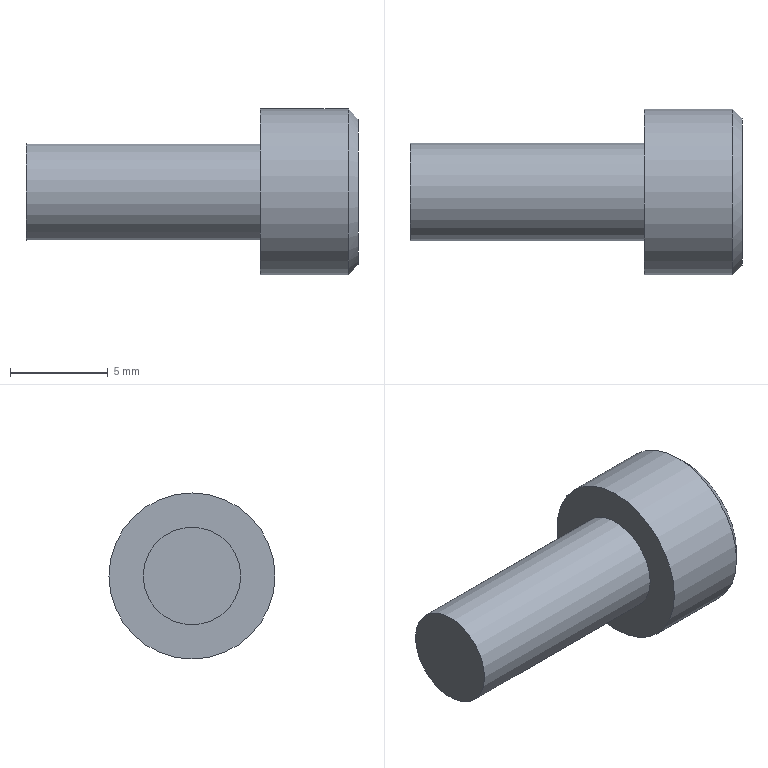Part | NX | features 5003_313_CB5-12 2 | 1 solid | 19 faces | box 17 x 8.5 x 8.5 mm | volume 476.463 mm3 | plane 15 | cylinder 2 | cone 2 | commonest cylinder face diameters 5 x1 8.5 x1
STEP:
#1=CARTESIAN_POINT('',(228.825,-163.25,-78.));
#2=VERTEX_POINT('',#1);
#3=CARTESIAN_POINT('',(228.825,-167.,-78.));
#4=DIRECTION('',(-1.,0.,0.));
#5=DIRECTION('',(0.,1.,0.));
#6=AXIS2_PLACEMENT_3D('',#3,#4,#5);
#7=CIRCLE('',#6,3.75);
#8=EDGE_CURVE('',#2,#2,#7,.F.);
#9=ORIENTED_EDGE('',*,*,#8,.T.);
#10=EDGE_LOOP('',(#9));
#11=FACE_BOUND('',#10,.T.);
#12=CARTESIAN_POINT('',(228.825,-167.,-75.691));
#13=VERTEX_POINT('',#12);
#14=CARTESIAN_POINT('',(228.825,-169.,-76.845));
#15=VERTEX_POINT('',#14);
#16=CARTESIAN_POINT('',(228.825,-167.,-75.691));
#17=DIRECTION('',(0.,-0.866,-0.5));
#18=VECTOR('',#17,1000.);
#19=LINE('',#16,#18);
#20=EDGE_CURVE('',#13,#15,#19,.T.);
#21=ORIENTED_EDGE('',*,*,#20,.F.);
#22=CARTESIAN_POINT('',(228.825,-165.,-76.845));
#23=VERTEX_POINT('',#22);
#24=CARTESIAN_POINT('',(228.825,-165.,-76.845));
#25=DIRECTION('',(0.,-0.866,0.5));
#26=VECTOR('',#25,1000.);
#27=LINE('',#24,#26);
#28=EDGE_CURVE('',#23,#13,#27,.T.);
#29=ORIENTED_EDGE('',*,*,#28,.F.);
#30=CARTESIAN_POINT('',(228.825,-165.,-79.155));
#31=VERTEX_POINT('',#30);
#32=CARTESIAN_POINT('',(228.825,-165.,-79.155));
#33=DIRECTION('',(0.,0.,1.));
#34=VECTOR('',#33,1000.);
#35=LINE('',#32,#34);
#36=EDGE_CURVE('',#31,#23,#35,.T.);
#37=ORIENTED_EDGE('',*,*,#36,.F.);
#38=CARTESIAN_POINT('',(228.825,-167.,-80.309));
#39=VERTEX_POINT('',#38);
#40=CARTESIAN_POINT('',(228.825,-167.,-80.309));
#41=DIRECTION('',(0.,0.866,0.5));
#42=VECTOR('',#41,1000.);
#43=LINE('',#40,#42);
#44=EDGE_CURVE('',#39,#31,#43,.T.);
#45=ORIENTED_EDGE('',*,*,#44,.F.);
#46=CARTESIAN_POINT('',(228.825,-169.,-79.155));
#47=VERTEX_POINT('',#46);
#48=CARTESIAN_POINT('',(228.825,-169.,-79.155));
#49=DIRECTION('',(0.,0.866,-0.5));
#50=VECTOR('',#49,1000.);
#51=LINE('',#48,#50);
#52=EDGE_CURVE('',#47,#39,#51,.T.);
#53=ORIENTED_EDGE('',*,*,#52,.F.);
#54=CARTESIAN_POINT('',(228.825,-169.,-76.845));
#55=DIRECTION('',(0.,0.,-1.));
#56=VECTOR('',#55,1000.);
#57=LINE('',#54,#56);
#58=EDGE_CURVE('',#15,#47,#57,.T.);
#59=ORIENTED_EDGE('',*,*,#58,.F.);
#60=EDGE_LOOP('',(#21,#29,#37,#45,#53,#59));
#61=FACE_BOUND('',#60,.T.);
#62=CARTESIAN_POINT('',(228.825,-167.,-82.25));
#63=DIRECTION('',(-1.,0.,0.));
#64=DIRECTION('',(0.,1.,0.));
#65=AXIS2_PLACEMENT_3D('',#62,#63,#64);
#66=PLANE('',#65);
#67=ADVANCED_FACE('',(#11,#61),#66,.F.);
#68=CARTESIAN_POINT('',(211.825,-169.5,-78.));
#69=VERTEX_POINT('',#68);
#70=CARTESIAN_POINT('',(211.825,-167.,-78.));
#71=DIRECTION('',(1.,0.,0.));
#72=DIRECTION('',(0.,-1.,0.));
#73=AXIS2_PLACEMENT_3D('',#70,#71,#72);
#74=CIRCLE('',#73,2.5);
#75=EDGE_CURVE('',#69,#69,#74,.T.);
#76=ORIENTED_EDGE('',*,*,#75,.F.);
#77=EDGE_LOOP('',(#76));
#78=FACE_BOUND('',#77,.T.);
#79=CARTESIAN_POINT('',(211.825,-167.,-78.));
#80=DIRECTION('',(1.,0.,0.));
#81=DIRECTION('',(0.,-1.,0.));
#82=AXIS2_PLACEMENT_3D('',#79,#80,#81);
#83=PLANE('',#82);
#84=ADVANCED_FACE('',(#78),#83,.F.);
#85=CARTESIAN_POINT('',(223.825,-169.5,-78.));
#86=VERTEX_POINT('',#85);
#87=CARTESIAN_POINT('',(223.825,-167.,-78.));
#88=DIRECTION('',(1.,0.,0.));
#89=DIRECTION('',(0.,-1.,0.));
#90=AXIS2_PLACEMENT_3D('',#87,#88,#89);
#91=CIRCLE('',#90,2.5);
#92=EDGE_CURVE('',#86,#86,#91,.T.);
#93=ORIENTED_EDGE('',*,*,#92,.F.);
#94=EDGE_LOOP('',(#93));
#95=FACE_BOUND('',#94,.T.);
#96=ORIENTED_EDGE('',*,*,#75,.T.);
#97=EDGE_LOOP('',(#96));
#98=FACE_BOUND('',#97,.T.);
#99=CARTESIAN_POINT('',(228.825,-167.,-78.));
#100=DIRECTION('',(1.,0.,0.));
#101=DIRECTION('',(0.,-1.,0.));
#102=AXIS2_PLACEMENT_3D('',#99,#100,#101);
#103=CYLINDRICAL_SURFACE('',#102,2.5);
#104=ADVANCED_FACE('',(#95,#98),#103,.T.);
#105=CARTESIAN_POINT('',(223.825,-171.25,-78.));
#106=VERTEX_POINT('',#105);
#107=CARTESIAN_POINT('',(223.825,-167.,-78.));
#108=DIRECTION('',(1.,0.,0.));
#109=DIRECTION('',(0.,-1.,0.));
#110=AXIS2_PLACEMENT_3D('',#107,#108,#109);
#111=CIRCLE('',#110,4.25);
#112=EDGE_CURVE('',#106,#106,#111,.T.);
#113=ORIENTED_EDGE('',*,*,#112,.F.);
#114=EDGE_LOOP('',(#113));
#115=FACE_BOUND('',#114,.T.);
#116=ORIENTED_EDGE('',*,*,#92,.T.);
#117=EDGE_LOOP('',(#116));
#118=FACE_BOUND('',#117,.T.);
#119=CARTESIAN_POINT('',(223.825,-167.,-80.5));
#120=DIRECTION('',(1.,0.,0.));
#121=DIRECTION('',(0.,-1.,0.));
#122=AXIS2_PLACEMENT_3D('',#119,#120,#121);
#123=PLANE('',#122);
#124=ADVANCED_FACE('',(#115,#118),#123,.F.);
#125=CARTESIAN_POINT('',(228.325,-162.75,-78.));
#126=VERTEX_POINT('',#125);
#127=CARTESIAN_POINT('',(228.325,-167.,-78.));
#128=DIRECTION('',(-1.,0.,0.));
#129=DIRECTION('',(0.,1.,0.));
#130=AXIS2_PLACEMENT_3D('',#127,#128,#129);
#131=CIRCLE('',#130,4.25);
#132=EDGE_CURVE('',#126,#126,#131,.T.);
#133=ORIENTED_EDGE('',*,*,#132,.T.);
#134=EDGE_LOOP('',(#133));
#135=FACE_BOUND('',#134,.T.);
#136=ORIENTED_EDGE('',*,*,#112,.T.);
#137=EDGE_LOOP('',(#136));
#138=FACE_BOUND('',#137,.T.);
#139=CARTESIAN_POINT('',(228.825,-167.,-78.));
#140=DIRECTION('',(1.,0.,0.));
#141=DIRECTION('',(0.,-1.,0.));
#142=AXIS2_PLACEMENT_3D('',#139,#140,#141);
#143=CYLINDRICAL_SURFACE('',#142,4.25);
#144=ADVANCED_FACE('',(#135,#138),#143,.T.);
#145=ORIENTED_EDGE('',*,*,#132,.F.);
#146=EDGE_LOOP('',(#145));
#147=FACE_BOUND('',#146,.T.);
#148=ORIENTED_EDGE('',*,*,#8,.F.);
#149=EDGE_LOOP('',(#148));
#150=FACE_BOUND('',#149,.T.);
#151=CARTESIAN_POINT('',(228.825,-167.,-78.));
#152=DIRECTION('',(-1.,0.,0.));
#153=DIRECTION('',(0.,1.,0.));
#154=AXIS2_PLACEMENT_3D('',#151,#152,#153);
#155=CONICAL_SURFACE('',#154,3.75,0.7854);
#156=ADVANCED_FACE('',(#147,#150),#155,.T.);
#157=CARTESIAN_POINT('',(226.325,-165.,-76.845));
#158=VERTEX_POINT('',#157);
#159=CARTESIAN_POINT('',(226.325,-166.,-76.268));
#160=VERTEX_POINT('',#159);
#161=CARTESIAN_POINT('',(226.325,-165.,-76.845));
#162=DIRECTION('',(0.,-0.866,0.5));
#163=VECTOR('',#162,1000.);
#164=LINE('',#161,#163);
#165=EDGE_CURVE('',#158,#160,#164,.T.);
#166=ORIENTED_EDGE('',*,*,#165,.F.);
#167=CARTESIAN_POINT('',(226.325,-165.,-76.845));
#168=DIRECTION('',(1.,0.,0.));
#169=VECTOR('',#168,1000.);
#170=LINE('',#167,#169);
#171=EDGE_CURVE('',#158,#23,#170,.T.);
#172=ORIENTED_EDGE('',*,*,#171,.T.);
#173=ORIENTED_EDGE('',*,*,#28,.T.);
#174=CARTESIAN_POINT('',(226.325,-167.,-75.691));
#175=VERTEX_POINT('',#174);
#176=CARTESIAN_POINT('',(226.325,-167.,-75.691));
#177=DIRECTION('',(1.,0.,0.));
#178=VECTOR('',#177,1000.);
#179=LINE('',#176,#178);
#180=EDGE_CURVE('',#175,#13,#179,.T.);
#181=ORIENTED_EDGE('',*,*,#180,.F.);
#182=CARTESIAN_POINT('',(226.325,-165.,-76.845));
#183=DIRECTION('',(0.,-0.866,0.5));
#184=VECTOR('',#183,1000.);
#185=LINE('',#182,#184);
#186=EDGE_CURVE('',#160,#175,#185,.T.);
#187=ORIENTED_EDGE('',*,*,#186,.F.);
#188=EDGE_LOOP('',(#166,#172,#173,#181,#187));
#189=FACE_BOUND('',#188,.T.);
#190=CARTESIAN_POINT('',(226.325,-165.,-76.845));
#191=DIRECTION('',(0.,0.5,0.866));
#192=DIRECTION('',(0.,0.866,-0.5));
#193=AXIS2_PLACEMENT_3D('',#190,#191,#192);
#194=PLANE('',#193);
#195=ADVANCED_FACE('',(#189),#194,.F.);
#196=CARTESIAN_POINT('',(226.325,-165.,-79.155));
#197=VERTEX_POINT('',#196);
#198=CARTESIAN_POINT('',(226.325,-165.,-78.));
#199=VERTEX_POINT('',#198);
#200=CARTESIAN_POINT('',(226.325,-165.,-79.155));
#201=DIRECTION('',(0.,0.,1.));
#202=VECTOR('',#201,1000.);
#203=LINE('',#200,#202);
#204=EDGE_CURVE('',#197,#199,#203,.T.);
#205=ORIENTED_EDGE('',*,*,#204,.F.);
#206=CARTESIAN_POINT('',(226.325,-165.,-79.155));
#207=DIRECTION('',(1.,0.,0.));
#208=VECTOR('',#207,1000.);
#209=LINE('',#206,#208);
#210=EDGE_CURVE('',#197,#31,#209,.T.);
#211=ORIENTED_EDGE('',*,*,#210,.T.);
#212=ORIENTED_EDGE('',*,*,#36,.T.);
#213=ORIENTED_EDGE('',*,*,#171,.F.);
#214=CARTESIAN_POINT('',(226.325,-165.,-79.155));
#215=DIRECTION('',(0.,0.,1.));
#216=VECTOR('',#215,1000.);
#217=LINE('',#214,#216);
#218=EDGE_CURVE('',#199,#158,#217,.T.);
#219=ORIENTED_EDGE('',*,*,#218,.F.);
#220=EDGE_LOOP('',(#205,#211,#212,#213,#219));
#221=FACE_BOUND('',#220,.T.);
#222=CARTESIAN_POINT('',(226.325,-165.,-79.155));
#223=DIRECTION('',(0.,1.,0.));
#224=DIRECTION('',(1.,0.,0.));
#225=AXIS2_PLACEMENT_3D('',#222,#223,#224);
#226=PLANE('',#225);
#227=ADVANCED_FACE('',(#221),#226,.F.);
#228=CARTESIAN_POINT('',(226.325,-167.,-80.309));
#229=VERTEX_POINT('',#228);
#230=CARTESIAN_POINT('',(226.325,-166.,-79.732));
#231=VERTEX_POINT('',#230);
#232=CARTESIAN_POINT('',(226.325,-167.,-80.309));
#233=DIRECTION('',(0.,0.866,0.5));
#234=VECTOR('',#233,1000.);
#235=LINE('',#232,#234);
#236=EDGE_CURVE('',#229,#231,#235,.T.);
#237=ORIENTED_EDGE('',*,*,#236,.F.);
#238=CARTESIAN_POINT('',(226.325,-167.,-80.309));
#239=DIRECTION('',(1.,0.,0.));
#240=VECTOR('',#239,1000.);
#241=LINE('',#238,#240);
#242=EDGE_CURVE('',#229,#39,#241,.T.);
#243=ORIENTED_EDGE('',*,*,#242,.T.);
#244=ORIENTED_EDGE('',*,*,#44,.T.);
#245=ORIENTED_EDGE('',*,*,#210,.F.);
#246=CARTESIAN_POINT('',(226.325,-167.,-80.309));
#247=DIRECTION('',(0.,0.866,0.5));
#248=VECTOR('',#247,1000.);
#249=LINE('',#246,#248);
#250=EDGE_CURVE('',#231,#197,#249,.T.);
#251=ORIENTED_EDGE('',*,*,#250,.F.);
#252=EDGE_LOOP('',(#237,#243,#244,#245,#251));
#253=FACE_BOUND('',#252,.T.);
#254=CARTESIAN_POINT('',(226.325,-167.,-80.309));
#255=DIRECTION('',(0.,0.5,-0.866));
#256=DIRECTION('',(0.,-0.866,-0.5));
#257=AXIS2_PLACEMENT_3D('',#254,#255,#256);
#258=PLANE('',#257);
#259=ADVANCED_FACE('',(#253),#258,.F.);
#260=CARTESIAN_POINT('',(226.325,-169.,-79.155));
#261=VERTEX_POINT('',#260);
#262=CARTESIAN_POINT('',(226.325,-168.,-79.732));
#263=VERTEX_POINT('',#262);
#264=CARTESIAN_POINT('',(226.325,-169.,-79.155));
#265=DIRECTION('',(0.,0.866,-0.5));
#266=VECTOR('',#265,1000.);
#267=LINE('',#264,#266);
#268=EDGE_CURVE('',#261,#263,#267,.T.);
#269=ORIENTED_EDGE('',*,*,#268,.F.);
#270=CARTESIAN_POINT('',(226.325,-169.,-79.155));
#271=DIRECTION('',(1.,0.,0.));
#272=VECTOR('',#271,1000.);
#273=LINE('',#270,#272);
#274=EDGE_CURVE('',#261,#47,#273,.T.);
#275=ORIENTED_EDGE('',*,*,#274,.T.);
#276=ORIENTED_EDGE('',*,*,#52,.T.);
#277=ORIENTED_EDGE('',*,*,#242,.F.);
#278=CARTESIAN_POINT('',(226.325,-169.,-79.155));
#279=DIRECTION('',(0.,0.866,-0.5));
#280=VECTOR('',#279,1000.);
#281=LINE('',#278,#280);
#282=EDGE_CURVE('',#263,#229,#281,.T.);
#283=ORIENTED_EDGE('',*,*,#282,.F.);
#284=EDGE_LOOP('',(#269,#275,#276,#277,#283));
#285=FACE_BOUND('',#284,.T.);
#286=CARTESIAN_POINT('',(226.325,-169.,-79.155));
#287=DIRECTION('',(0.,-0.5,-0.866));
#288=DIRECTION('',(0.,-0.866,0.5));
#289=AXIS2_PLACEMENT_3D('',#286,#287,#288);
#290=PLANE('',#289);
#291=ADVANCED_FACE('',(#285),#290,.F.);
#292=CARTESIAN_POINT('',(226.325,-169.,-76.845));
#293=VERTEX_POINT('',#292);
#294=CARTESIAN_POINT('',(226.325,-169.,-78.));
#295=VERTEX_POINT('',#294);
#296=CARTESIAN_POINT('',(226.325,-169.,-76.845));
#297=DIRECTION('',(0.,0.,-1.));
#298=VECTOR('',#297,1000.);
#299=LINE('',#296,#298);
#300=EDGE_CURVE('',#293,#295,#299,.T.);
#301=ORIENTED_EDGE('',*,*,#300,.F.);
#302=CARTESIAN_POINT('',(226.325,-169.,-76.845));
#303=DIRECTION('',(1.,0.,0.));
#304=VECTOR('',#303,1000.);
#305=LINE('',#302,#304);
#306=EDGE_CURVE('',#293,#15,#305,.T.);
#307=ORIENTED_EDGE('',*,*,#306,.T.);
#308=ORIENTED_EDGE('',*,*,#58,.T.);
#309=ORIENTED_EDGE('',*,*,#274,.F.);
#310=CARTESIAN_POINT('',(226.325,-169.,-76.845));
#311=DIRECTION('',(0.,0.,-1.));
#312=VECTOR('',#311,1000.);
#313=LINE('',#310,#312);
#314=EDGE_CURVE('',#295,#261,#313,.T.);
#315=ORIENTED_EDGE('',*,*,#314,.F.);
#316=EDGE_LOOP('',(#301,#307,#308,#309,#315));
#317=FACE_BOUND('',#316,.T.);
#318=CARTESIAN_POINT('',(226.325,-169.,-76.845));
#319=DIRECTION('',(0.,-1.,0.));
#320=DIRECTION('',(0.,0.,1.));
#321=AXIS2_PLACEMENT_3D('',#318,#319,#320);
#322=PLANE('',#321);
#323=ADVANCED_FACE('',(#317),#322,.F.);
#324=CARTESIAN_POINT('',(226.325,-168.,-76.268));
#325=VERTEX_POINT('',#324);
#326=CARTESIAN_POINT('',(226.325,-167.,-75.691));
#327=DIRECTION('',(0.,-0.866,-0.5));
#328=VECTOR('',#327,1000.);
#329=LINE('',#326,#328);
#330=EDGE_CURVE('',#175,#325,#329,.T.);
#331=ORIENTED_EDGE('',*,*,#330,.F.);
#332=ORIENTED_EDGE('',*,*,#180,.T.);
#333=ORIENTED_EDGE('',*,*,#20,.T.);
#334=ORIENTED_EDGE('',*,*,#306,.F.);
#335=CARTESIAN_POINT('',(226.325,-167.,-75.691));
#336=DIRECTION('',(0.,-0.866,-0.5));
#337=VECTOR('',#336,1000.);
#338=LINE('',#335,#337);
#339=EDGE_CURVE('',#325,#293,#338,.T.);
#340=ORIENTED_EDGE('',*,*,#339,.F.);
#341=EDGE_LOOP('',(#331,#332,#333,#334,#340));
#342=FACE_BOUND('',#341,.T.);
#343=CARTESIAN_POINT('',(226.325,-167.,-75.691));
#344=DIRECTION('',(0.,-0.5,0.866));
#345=DIRECTION('',(0.,0.866,0.5));
#346=AXIS2_PLACEMENT_3D('',#343,#344,#345);
#347=PLANE('',#346);
#348=ADVANCED_FACE('',(#342),#347,.F.);
#349=ORIENTED_EDGE('',*,*,#314,.T.);
#350=ORIENTED_EDGE('',*,*,#268,.T.);
#351=CARTESIAN_POINT('',(226.325,-167.,-78.));
#352=DIRECTION('',(1.,0.,0.));
#353=DIRECTION('',(0.,0.,1.));
#354=AXIS2_PLACEMENT_3D('',#351,#352,#353);
#355=CIRCLE('',#354,2.);
#356=EDGE_CURVE('',#295,#263,#355,.T.);
#357=ORIENTED_EDGE('',*,*,#356,.F.);
#358=EDGE_LOOP('',(#349,#350,#357));
#359=FACE_BOUND('',#358,.T.);
#360=CARTESIAN_POINT('',(226.325,-167.,-78.));
#361=DIRECTION('',(1.,0.,0.));
#362=DIRECTION('',(0.,-1.,0.));
#363=AXIS2_PLACEMENT_3D('',#360,#361,#362);
#364=PLANE('',#363);
#365=ADVANCED_FACE('',(#359),#364,.T.);
#366=ORIENTED_EDGE('',*,*,#282,.T.);
#367=ORIENTED_EDGE('',*,*,#236,.T.);
#368=CARTESIAN_POINT('',(226.325,-167.,-78.));
#369=DIRECTION('',(1.,0.,0.));
#370=DIRECTION('',(0.,0.,1.));
#371=AXIS2_PLACEMENT_3D('',#368,#369,#370);
#372=CIRCLE('',#371,2.);
#373=EDGE_CURVE('',#263,#231,#372,.T.);
#374=ORIENTED_EDGE('',*,*,#373,.F.);
#375=EDGE_LOOP('',(#366,#367,#374));
#376=FACE_BOUND('',#375,.T.);
#377=CARTESIAN_POINT('',(226.325,-167.,-78.));
#378=DIRECTION('',(1.,0.,0.));
#379=DIRECTION('',(0.,-1.,0.));
#380=AXIS2_PLACEMENT_3D('',#377,#378,#379);
#381=PLANE('',#380);
#382=ADVANCED_FACE('',(#376),#381,.T.);
#383=ORIENTED_EDGE('',*,*,#250,.T.);
#384=ORIENTED_EDGE('',*,*,#204,.T.);
#385=CARTESIAN_POINT('',(226.325,-167.,-78.));
#386=DIRECTION('',(1.,0.,0.));
#387=DIRECTION('',(0.,0.,1.));
#388=AXIS2_PLACEMENT_3D('',#385,#386,#387);
#389=CIRCLE('',#388,2.);
#390=EDGE_CURVE('',#231,#199,#389,.T.);
#391=ORIENTED_EDGE('',*,*,#390,.F.);
#392=EDGE_LOOP('',(#383,#384,#391));
#393=FACE_BOUND('',#392,.T.);
#394=CARTESIAN_POINT('',(226.325,-167.,-78.));
#395=DIRECTION('',(1.,0.,0.));
#396=DIRECTION('',(0.,-1.,0.));
#397=AXIS2_PLACEMENT_3D('',#394,#395,#396);
#398=PLANE('',#397);
#399=ADVANCED_FACE('',(#393),#398,.T.);
#400=ORIENTED_EDGE('',*,*,#218,.T.);
#401=ORIENTED_EDGE('',*,*,#165,.T.);
#402=CARTESIAN_POINT('',(226.325,-167.,-78.));
#403=DIRECTION('',(1.,0.,0.));
#404=DIRECTION('',(0.,0.,1.));
#405=AXIS2_PLACEMENT_3D('',#402,#403,#404);
#406=CIRCLE('',#405,2.);
#407=EDGE_CURVE('',#199,#160,#406,.T.);
#408=ORIENTED_EDGE('',*,*,#407,.F.);
#409=EDGE_LOOP('',(#400,#401,#408));
#410=FACE_BOUND('',#409,.T.);
#411=CARTESIAN_POINT('',(226.325,-167.,-78.));
#412=DIRECTION('',(1.,0.,0.));
#413=DIRECTION('',(0.,-1.,0.));
#414=AXIS2_PLACEMENT_3D('',#411,#412,#413);
#415=PLANE('',#414);
#416=ADVANCED_FACE('',(#410),#415,.T.);
#417=ORIENTED_EDGE('',*,*,#186,.T.);
#418=ORIENTED_EDGE('',*,*,#330,.T.);
#419=CARTESIAN_POINT('',(226.325,-167.,-78.));
#420=DIRECTION('',(1.,0.,0.));
#421=DIRECTION('',(0.,0.,1.));
#422=AXIS2_PLACEMENT_3D('',#419,#420,#421);
#423=CIRCLE('',#422,2.);
#424=EDGE_CURVE('',#160,#325,#423,.T.);
#425=ORIENTED_EDGE('',*,*,#424,.F.);
#426=EDGE_LOOP('',(#417,#418,#425));
#427=FACE_BOUND('',#426,.T.);
#428=CARTESIAN_POINT('',(226.325,-167.,-78.));
#429=DIRECTION('',(1.,0.,0.));
#430=DIRECTION('',(0.,-1.,0.));
#431=AXIS2_PLACEMENT_3D('',#428,#429,#430);
#432=PLANE('',#431);
#433=ADVANCED_FACE('',(#427),#432,.T.);
#434=ORIENTED_EDGE('',*,*,#339,.T.);
#435=ORIENTED_EDGE('',*,*,#300,.T.);
#436=CARTESIAN_POINT('',(226.325,-167.,-78.));
#437=DIRECTION('',(1.,0.,0.));
#438=DIRECTION('',(0.,0.,1.));
#439=AXIS2_PLACEMENT_3D('',#436,#437,#438);
#440=CIRCLE('',#439,2.);
#441=EDGE_CURVE('',#325,#295,#440,.T.);
#442=ORIENTED_EDGE('',*,*,#441,.F.);
#443=EDGE_LOOP('',(#434,#435,#442));
#444=FACE_BOUND('',#443,.T.);
#445=CARTESIAN_POINT('',(226.325,-167.,-78.));
#446=DIRECTION('',(1.,0.,0.));
#447=DIRECTION('',(0.,-1.,0.));
#448=AXIS2_PLACEMENT_3D('',#445,#446,#447);
#449=PLANE('',#448);
#450=ADVANCED_FACE('',(#444),#449,.T.);
#451=ORIENTED_EDGE('',*,*,#441,.T.);
#452=ORIENTED_EDGE('',*,*,#356,.T.);
#453=ORIENTED_EDGE('',*,*,#373,.T.);
#454=ORIENTED_EDGE('',*,*,#390,.T.);
#455=ORIENTED_EDGE('',*,*,#407,.T.);
#456=ORIENTED_EDGE('',*,*,#424,.T.);
#457=EDGE_LOOP('',(#451,#452,#453,#454,#455,#456));
#458=FACE_BOUND('',#457,.T.);
#459=CARTESIAN_POINT('',(225.123,-167.,-78.));
#460=VERTEX_POINT('',#459);
#461=VERTEX_LOOP('',#460);
#462=FACE_BOUND('',#461,.T.);
#463=CARTESIAN_POINT('',(225.123,-167.,-78.));
#464=DIRECTION('',(1.,0.,0.));
#465=DIRECTION('',(0.,0.,1.));
#466=AXIS2_PLACEMENT_3D('',#463,#464,#465);
#467=CONICAL_SURFACE('',#466,0.,1.03);
#468=ADVANCED_FACE('',(#458,#462),#467,.F.);
#469=CLOSED_SHELL('',(#67,#84,#104,#124,#144,#156,#195,#227,#259,#291,#323,#348,#365,#382,#399,#416,#433,#450,#468));
#470=MANIFOLD_SOLID_BREP('',#469);
#471=(LENGTH_UNIT()NAMED_UNIT(*)SI_UNIT(.MILLI.,.METRE.));
#472=UNCERTAINTY_MEASURE_WITH_UNIT(LENGTH_MEASURE(0.00001),#471,'','');
#473=(NAMED_UNIT(*)PLANE_ANGLE_UNIT()SI_UNIT($,.RADIAN.));
#474=(NAMED_UNIT(*)SI_UNIT($,.STERADIAN.)SOLID_ANGLE_UNIT());
#475=(GEOMETRIC_REPRESENTATION_CONTEXT(3)GLOBAL_UNCERTAINTY_ASSIGNED_CONTEXT((#472))GLOBAL_UNIT_ASSIGNED_CONTEXT((#471,#473,#474))REPRESENTATION_CONTEXT('',''));
#476=ADVANCED_BREP_SHAPE_REPRESENTATION('',(#470),#475);